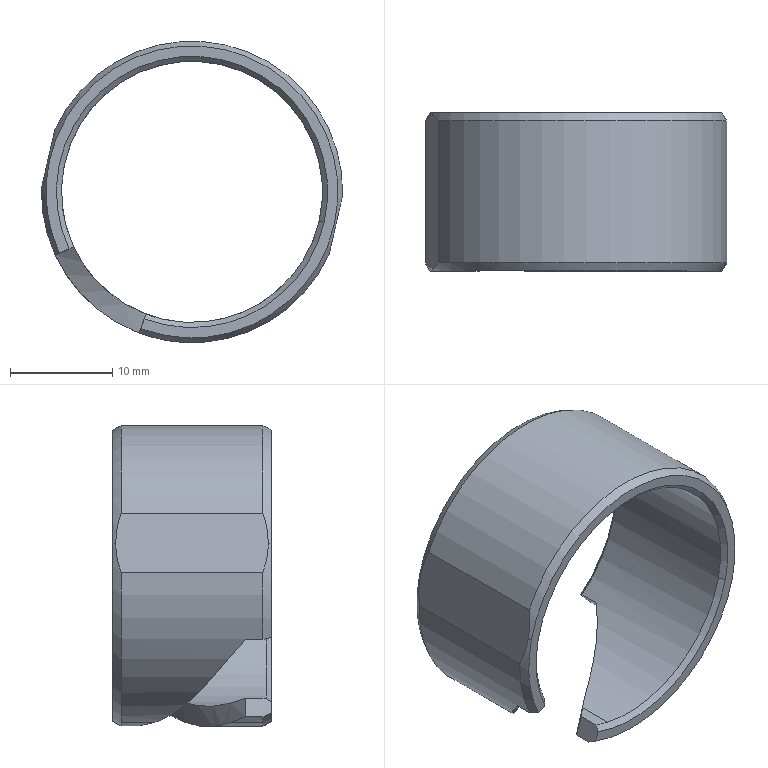Part | SolidWorks | features BaseBody 1 | 1 solid | 31 faces | box 29.5 x 15.5 x 29.5 mm | volume 2238 mm3 | cone 12 | cylinder 9 | plane 8 | spline 2 | commonest cylinder face diameters 29.5 x5 25.55 x4
STEP:
#1=CARTESIAN_POINT('',(1955.861,229.,865.451));
#2=VERTEX_POINT('',#1);
#3=CARTESIAN_POINT('',(1940.549,229.,855.861));
#4=VERTEX_POINT('',#3);
#5=CARTESIAN_POINT('',(1953.,229.,853.));
#6=DIRECTION('',(0.,-1.,0.));
#7=DIRECTION('',(0.2239,0.,0.9746));
#8=AXIS2_PLACEMENT_3D('',#5,#6,#7);
#9=CIRCLE('',#8,12.775);
#10=EDGE_CURVE('',#2,#4,#9,.T.);
#11=ORIENTED_EDGE('',*,*,#10,.T.);
#12=CARTESIAN_POINT('',(1940.062,229.5,855.973));
#13=VERTEX_POINT('',#12);
#14=CARTESIAN_POINT('',(1940.306,229.25,855.917));
#15=DIRECTION('',(-0.6891,0.7071,0.1583));
#16=VECTOR('',#15,1000.);
#17=LINE('',#14,#16);
#18=EDGE_CURVE('',#4,#13,#17,.T.);
#19=ORIENTED_EDGE('',*,*,#18,.T.);
#20=CARTESIAN_POINT('',(1955.973,229.5,865.938));
#21=VERTEX_POINT('',#20);
#22=CARTESIAN_POINT('',(1953.,229.5,853.));
#23=DIRECTION('',(0.,-1.,0.));
#24=DIRECTION('',(0.2239,0.,0.9746));
#25=AXIS2_PLACEMENT_3D('',#22,#23,#24);
#26=CIRCLE('',#25,13.275);
#27=EDGE_CURVE('',#21,#13,#26,.T.);
#28=ORIENTED_EDGE('',*,*,#27,.F.);
#29=CARTESIAN_POINT('',(1955.973,229.5,865.938));
#30=DIRECTION('',(-0.1583,-0.7071,-0.6891));
#31=VECTOR('',#30,1000.);
#32=LINE('',#29,#31);
#33=EDGE_CURVE('',#21,#2,#32,.T.);
#34=ORIENTED_EDGE('',*,*,#33,.T.);
#35=EDGE_LOOP('',(#11,#19,#28,#34));
#36=FACE_OUTER_BOUND('',#35,.T.);
#37=CARTESIAN_POINT('',(1953.,229.25,853.));
#38=DIRECTION('',(0.,1.,0.));
#39=DIRECTION('',(-0.9746,0.,0.2239));
#40=AXIS2_PLACEMENT_3D('',#37,#38,#39);
#41=CONICAL_SURFACE('',#40,13.025,0.7854);
#42=ADVANCED_FACE('',(#36),#41,.F.);
#43=CARTESIAN_POINT('',(1950.139,225.489,840.549));
#44=VERTEX_POINT('',#43);
#45=CARTESIAN_POINT('',(1941.412,216.5,847.623));
#46=VERTEX_POINT('',#45);
#47=CARTESIAN_POINT('',(1950.139,225.489,840.549));
#48=CARTESIAN_POINT('',(1949.226,224.707,840.759));
#49=CARTESIAN_POINT('',(1948.307,223.97,841.077));
#50=CARTESIAN_POINT('',(1946.969,222.878,841.727));
#51=CARTESIAN_POINT('',(1946.53,222.517,841.973));
#52=CARTESIAN_POINT('',(1945.691,221.804,842.51));
#53=CARTESIAN_POINT('',(1945.289,221.45,842.803));
#54=CARTESIAN_POINT('',(1944.523,220.739,843.43));
#55=CARTESIAN_POINT('',(1944.16,220.382,843.764));
#56=CARTESIAN_POINT('',(1943.477,219.655,844.47));
#57=CARTESIAN_POINT('',(1943.156,219.284,844.843));
#58=CARTESIAN_POINT('',(1942.27,218.141,845.999));
#59=CARTESIAN_POINT('',(1941.789,217.352,846.811));
#60=CARTESIAN_POINT('',(1941.412,216.5,847.623));
#61=B_SPLINE_CURVE_WITH_KNOTS('',3,(#47,#48,#49,#50,#51,#52,#53,#54,#55,#56,#57,#58,#59,#60),.UNSPECIFIED.,.F.,.F.,(4,2,2,2,2,2,4),(0.002262,0.005917,0.007745,0.009573,0.0114,0.01323,0.01689),.UNSPECIFIED.);
#62=EDGE_CURVE('',#44,#46,#61,.T.);
#63=ORIENTED_EDGE('',*,*,#62,.F.);
#64=CARTESIAN_POINT('',(1950.139,229.,840.549));
#65=VERTEX_POINT('',#64);
#66=CARTESIAN_POINT('',(1950.139,214.,840.549));
#67=DIRECTION('',(0.,1.,0.));
#68=VECTOR('',#67,1000.);
#69=LINE('',#66,#68);
#70=EDGE_CURVE('',#44,#65,#69,.T.);
#71=ORIENTED_EDGE('',*,*,#70,.T.);
#72=CARTESIAN_POINT('',(1953.,229.,853.));
#73=DIRECTION('',(0.,-1.,0.));
#74=DIRECTION('',(0.2239,0.,0.9746));
#75=AXIS2_PLACEMENT_3D('',#72,#73,#74);
#76=CIRCLE('',#75,12.775);
#77=EDGE_CURVE('',#4,#65,#76,.T.);
#78=ORIENTED_EDGE('',*,*,#77,.F.);
#79=ORIENTED_EDGE('',*,*,#10,.F.);
#80=CARTESIAN_POINT('',(1955.861,214.5,865.451));
#81=VERTEX_POINT('',#80);
#82=CARTESIAN_POINT('',(1955.861,214.5,865.451));
#83=DIRECTION('',(0.,1.,0.));
#84=VECTOR('',#83,1000.);
#85=LINE('',#82,#84);
#86=EDGE_CURVE('',#81,#2,#85,.T.);
#87=ORIENTED_EDGE('',*,*,#86,.F.);
#88=CARTESIAN_POINT('',(1941.412,214.5,847.623));
#89=VERTEX_POINT('',#88);
#90=CARTESIAN_POINT('',(1953.,214.5,853.));
#91=DIRECTION('',(0.,-1.,0.));
#92=DIRECTION('',(0.2239,0.,0.9746));
#93=AXIS2_PLACEMENT_3D('',#90,#91,#92);
#94=CIRCLE('',#93,12.775);
#95=EDGE_CURVE('',#81,#89,#94,.T.);
#96=ORIENTED_EDGE('',*,*,#95,.T.);
#97=CARTESIAN_POINT('',(1941.412,214.5,847.623));
#98=DIRECTION('',(0.,1.,0.));
#99=VECTOR('',#98,1000.);
#100=LINE('',#97,#99);
#101=EDGE_CURVE('',#89,#46,#100,.T.);
#102=ORIENTED_EDGE('',*,*,#101,.T.);
#103=EDGE_LOOP('',(#63,#71,#78,#79,#87,#96,#102));
#104=FACE_OUTER_BOUND('',#103,.T.);
#105=CARTESIAN_POINT('',(1953.,214.,853.));
#106=DIRECTION('',(0.,1.,0.));
#107=DIRECTION('',(-0.2239,0.,-0.9746));
#108=AXIS2_PLACEMENT_3D('',#105,#106,#107);
#109=CYLINDRICAL_SURFACE('',#108,12.775);
#110=ADVANCED_FACE('',(#104),#109,.F.);
#111=CARTESIAN_POINT('',(1939.075,229.5,856.2));
#112=VERTEX_POINT('',#111);
#113=CARTESIAN_POINT('',(1966.925,229.5,849.8));
#114=VERTEX_POINT('',#113);
#115=CARTESIAN_POINT('',(1953.,229.5,853.));
#116=DIRECTION('',(0.,1.,0.));
#117=DIRECTION('',(-0.09251,0.,-0.9957));
#118=AXIS2_PLACEMENT_3D('',#115,#116,#117);
#119=CIRCLE('',#118,14.288);
#120=EDGE_CURVE('',#112,#114,#119,.T.);
#121=ORIENTED_EDGE('',*,*,#120,.F.);
#122=CARTESIAN_POINT('',(1938.917,229.22,856.236));
#123=VERTEX_POINT('',#122);
#124=CARTESIAN_POINT('',(1938.85,229.1,856.251));
#125=DIRECTION('',(-0.4873,-0.866,0.112));
#126=VECTOR('',#125,1000.);
#127=LINE('',#124,#126);
#128=EDGE_CURVE('',#112,#123,#127,.T.);
#129=ORIENTED_EDGE('',*,*,#128,.T.);
#130=CARTESIAN_POINT('',(1939.58,228.7,859.12));
#131=VERTEX_POINT('',#130);
#132=CARTESIAN_POINT('',(1938.917,229.22,856.236));
#133=CARTESIAN_POINT('',(1939.145,229.22,857.227));
#134=CARTESIAN_POINT('',(1939.365,229.033,858.186));
#135=CARTESIAN_POINT('',(1939.58,228.7,859.12));
#136=B_SPLINE_CURVE_WITH_KNOTS('',3,(#132,#133,#134,#135),.UNSPECIFIED.,.F.,.F.,(4,4),(0.003005,0.006011),.UNSPECIFIED.);
#137=EDGE_CURVE('',#123,#131,#136,.T.);
#138=ORIENTED_EDGE('',*,*,#137,.T.);
#139=CARTESIAN_POINT('',(1967.746,228.7,852.649));
#140=VERTEX_POINT('',#139);
#141=CARTESIAN_POINT('',(1953.,228.7,853.));
#142=DIRECTION('',(0.,-1.,0.));
#143=DIRECTION('',(0.9997,0.,-0.02381));
#144=AXIS2_PLACEMENT_3D('',#141,#142,#143);
#145=CIRCLE('',#144,14.75);
#146=EDGE_CURVE('',#140,#131,#145,.T.);
#147=ORIENTED_EDGE('',*,*,#146,.F.);
#148=CARTESIAN_POINT('',(1967.083,229.22,849.764));
#149=VERTEX_POINT('',#148);
#150=CARTESIAN_POINT('',(1967.746,228.7,852.649));
#151=CARTESIAN_POINT('',(1967.531,229.033,851.715));
#152=CARTESIAN_POINT('',(1967.311,229.22,850.755));
#153=CARTESIAN_POINT('',(1967.083,229.22,849.764));
#154=B_SPLINE_CURVE_WITH_KNOTS('',3,(#150,#151,#152,#153),.UNSPECIFIED.,.F.,.F.,(4,4),(0.,0.003005),.UNSPECIFIED.);
#155=EDGE_CURVE('',#140,#149,#154,.T.);
#156=ORIENTED_EDGE('',*,*,#155,.T.);
#157=CARTESIAN_POINT('',(1967.15,229.1,849.749));
#158=DIRECTION('',(0.4873,-0.866,-0.112));
#159=VECTOR('',#158,1000.);
#160=LINE('',#157,#159);
#161=EDGE_CURVE('',#114,#149,#160,.T.);
#162=ORIENTED_EDGE('',*,*,#161,.F.);
#163=EDGE_LOOP('',(#121,#129,#138,#147,#156,#162));
#164=FACE_OUTER_BOUND('',#163,.T.);
#165=CARTESIAN_POINT('',(1953.,229.1,853.));
#166=DIRECTION('',(0.,-1.,0.));
#167=DIRECTION('',(0.9746,0.,-0.2239));
#168=AXIS2_PLACEMENT_3D('',#165,#166,#167);
#169=CONICAL_SURFACE('',#168,14.519,0.5236);
#170=ADVANCED_FACE('',(#164),#169,.T.);
#171=CARTESIAN_POINT('',(1962.036,229.5,841.932));
#172=VERTEX_POINT('',#171);
#173=CARTESIAN_POINT('',(1953.,229.5,853.));
#174=DIRECTION('',(0.,1.,0.));
#175=DIRECTION('',(-0.09251,0.,-0.9957));
#176=AXIS2_PLACEMENT_3D('',#173,#174,#175);
#177=CIRCLE('',#176,14.288);
#178=EDGE_CURVE('',#114,#172,#177,.T.);
#179=ORIENTED_EDGE('',*,*,#178,.F.);
#180=ORIENTED_EDGE('',*,*,#161,.T.);
#181=CARTESIAN_POINT('',(1966.42,228.7,846.88));
#182=VERTEX_POINT('',#181);
#183=CARTESIAN_POINT('',(1967.083,229.22,849.764));
#184=CARTESIAN_POINT('',(1966.855,229.22,848.773));
#185=CARTESIAN_POINT('',(1966.635,229.033,847.814));
#186=CARTESIAN_POINT('',(1966.42,228.7,846.88));
#187=B_SPLINE_CURVE_WITH_KNOTS('',3,(#183,#184,#185,#186),.UNSPECIFIED.,.F.,.F.,(4,4),(0.003005,0.006011),.UNSPECIFIED.);
#188=EDGE_CURVE('',#149,#182,#187,.T.);
#189=ORIENTED_EDGE('',*,*,#188,.T.);
#190=CARTESIAN_POINT('',(1962.328,228.7,841.574));
#191=VERTEX_POINT('',#190);
#192=CARTESIAN_POINT('',(1953.,228.7,853.));
#193=DIRECTION('',(0.,1.,0.));
#194=DIRECTION('',(0.9098,0.,-0.4149));
#195=AXIS2_PLACEMENT_3D('',#192,#193,#194);
#196=CIRCLE('',#195,14.75);
#197=EDGE_CURVE('',#182,#191,#196,.T.);
#198=ORIENTED_EDGE('',*,*,#197,.T.);
#199=CARTESIAN_POINT('',(1962.328,228.7,841.574));
#200=DIRECTION('',(-0.3162,0.866,0.3873));
#201=VECTOR('',#200,1000.);
#202=LINE('',#199,#201);
#203=EDGE_CURVE('',#191,#172,#202,.T.);
#204=ORIENTED_EDGE('',*,*,#203,.T.);
#205=EDGE_LOOP('',(#179,#180,#189,#198,#204));
#206=FACE_OUTER_BOUND('',#205,.T.);
#207=CARTESIAN_POINT('',(1953.,229.1,853.));
#208=DIRECTION('',(0.,-1.,0.));
#209=DIRECTION('',(0.9746,0.,-0.2239));
#210=AXIS2_PLACEMENT_3D('',#207,#208,#209);
#211=CONICAL_SURFACE('',#210,14.519,0.5236);
#212=ADVANCED_FACE('',(#206),#211,.T.);
#213=CARTESIAN_POINT('',(1949.697,225.489,838.625));
#214=VERTEX_POINT('',#213);
#215=CARTESIAN_POINT('',(1951.636,227.,838.313));
#216=VERTEX_POINT('',#215);
#217=CARTESIAN_POINT('',(1949.697,225.489,838.625));
#218=CARTESIAN_POINT('',(1950.348,225.972,838.475));
#219=CARTESIAN_POINT('',(1950.997,226.472,838.373));
#220=CARTESIAN_POINT('',(1951.636,227.,838.313));
#221=B_SPLINE_CURVE_WITH_KNOTS('',3,(#217,#218,#219,#220),.UNSPECIFIED.,.F.,.F.,(4,4),(0.01609,0.01854),.UNSPECIFIED.);
#222=EDGE_CURVE('',#214,#216,#221,.T.);
#223=ORIENTED_EDGE('',*,*,#222,.F.);
#224=CARTESIAN_POINT('',(1949.697,228.7,838.625));
#225=VERTEX_POINT('',#224);
#226=CARTESIAN_POINT('',(1949.697,214.,838.625));
#227=DIRECTION('',(0.,1.,0.));
#228=VECTOR('',#227,1000.);
#229=LINE('',#226,#228);
#230=EDGE_CURVE('',#214,#225,#229,.T.);
#231=ORIENTED_EDGE('',*,*,#230,.T.);
#232=CARTESIAN_POINT('',(1951.636,228.7,838.313));
#233=VERTEX_POINT('',#232);
#234=CARTESIAN_POINT('',(1953.,228.7,853.));
#235=DIRECTION('',(0.,-1.,0.));
#236=DIRECTION('',(-0.9997,0.,0.02381));
#237=AXIS2_PLACEMENT_3D('',#234,#235,#236);
#238=CIRCLE('',#237,14.75);
#239=EDGE_CURVE('',#225,#233,#238,.T.);
#240=ORIENTED_EDGE('',*,*,#239,.T.);
#241=CARTESIAN_POINT('',(1951.636,227.,838.313));
#242=DIRECTION('',(0.,1.,0.));
#243=VECTOR('',#242,1000.);
#244=LINE('',#241,#243);
#245=EDGE_CURVE('',#216,#233,#244,.T.);
#246=ORIENTED_EDGE('',*,*,#245,.F.);
#247=EDGE_LOOP('',(#223,#231,#240,#246));
#248=FACE_OUTER_BOUND('',#247,.T.);
#249=CARTESIAN_POINT('',(1953.,214.,853.));
#250=DIRECTION('',(0.,1.,0.));
#251=DIRECTION('',(-0.2239,0.,-0.9746));
#252=AXIS2_PLACEMENT_3D('',#249,#250,#251);
#253=CYLINDRICAL_SURFACE('',#252,14.75);
#254=ADVANCED_FACE('',(#248),#253,.T.);
#255=CARTESIAN_POINT('',(1966.42,214.8,846.88));
#256=VERTEX_POINT('',#255);
#257=CARTESIAN_POINT('',(1949.697,214.8,838.625));
#258=VERTEX_POINT('',#257);
#259=CARTESIAN_POINT('',(1953.,214.8,853.));
#260=DIRECTION('',(0.,1.,0.));
#261=DIRECTION('',(0.9098,0.,-0.4149));
#262=AXIS2_PLACEMENT_3D('',#259,#260,#261);
#263=CIRCLE('',#262,14.75);
#264=EDGE_CURVE('',#256,#258,#263,.T.);
#265=ORIENTED_EDGE('',*,*,#264,.T.);
#266=CARTESIAN_POINT('',(1949.697,218.011,838.625));
#267=VERTEX_POINT('',#266);
#268=CARTESIAN_POINT('',(1949.697,214.,838.625));
#269=DIRECTION('',(0.,1.,0.));
#270=VECTOR('',#269,1000.);
#271=LINE('',#268,#270);
#272=EDGE_CURVE('',#258,#267,#271,.T.);
#273=ORIENTED_EDGE('',*,*,#272,.T.);
#274=CARTESIAN_POINT('',(1962.328,227.,841.574));
#275=VERTEX_POINT('',#274);
#276=CARTESIAN_POINT('',(1962.328,227.,841.574));
#277=CARTESIAN_POINT('',(1961.515,226.136,840.911));
#278=CARTESIAN_POINT('',(1960.605,225.349,840.313));
#279=CARTESIAN_POINT('',(1959.117,224.219,839.567));
#280=CARTESIAN_POINT('',(1958.601,223.85,839.343));
#281=CARTESIAN_POINT('',(1957.533,223.121,838.952));
#282=CARTESIAN_POINT('',(1956.979,222.759,838.785));
#283=CARTESIAN_POINT('',(1955.309,221.691,838.387));
#284=CARTESIAN_POINT('',(1954.171,220.994,838.253));
#285=CARTESIAN_POINT('',(1952.468,219.913,838.249));
#286=CARTESIAN_POINT('',(1951.899,219.544,838.28));
#287=CARTESIAN_POINT('',(1950.778,218.79,838.407));
#288=CARTESIAN_POINT('',(1950.23,218.407,838.502));
#289=CARTESIAN_POINT('',(1949.697,218.011,838.625));
#290=B_SPLINE_CURVE_WITH_KNOTS('',3,(#276,#277,#278,#279,#280,#281,#282,#283,#284,#285,#286,#287,#288,#289),.UNSPECIFIED.,.F.,.F.,(4,2,2,2,2,2,4),(0.,0.004021,0.006032,0.008043,0.01206,0.01407,0.01609),.UNSPECIFIED.);
#291=EDGE_CURVE('',#275,#267,#290,.T.);
#292=ORIENTED_EDGE('',*,*,#291,.F.);
#293=CARTESIAN_POINT('',(1962.328,227.,841.574));
#294=DIRECTION('',(0.,1.,0.));
#295=VECTOR('',#294,1000.);
#296=LINE('',#293,#295);
#297=EDGE_CURVE('',#275,#191,#296,.T.);
#298=ORIENTED_EDGE('',*,*,#297,.T.);
#299=ORIENTED_EDGE('',*,*,#197,.F.);
#300=CARTESIAN_POINT('',(1966.42,214.8,846.88));
#301=DIRECTION('',(0.,1.,0.));
#302=VECTOR('',#301,1000.);
#303=LINE('',#300,#302);
#304=EDGE_CURVE('',#256,#182,#303,.T.);
#305=ORIENTED_EDGE('',*,*,#304,.F.);
#306=EDGE_LOOP('',(#265,#273,#292,#298,#299,#305));
#307=FACE_OUTER_BOUND('',#306,.T.);
#308=CARTESIAN_POINT('',(1953.,214.,853.));
#309=DIRECTION('',(0.,1.,0.));
#310=DIRECTION('',(-0.2239,0.,-0.9746));
#311=AXIS2_PLACEMENT_3D('',#308,#309,#310);
#312=CYLINDRICAL_SURFACE('',#311,14.75);
#313=ADVANCED_FACE('',(#307),#312,.T.);
#314=CARTESIAN_POINT('',(1950.139,214.5,840.549));
#315=VERTEX_POINT('',#314);
#316=CARTESIAN_POINT('',(1948.511,214.5,841.04));
#317=VERTEX_POINT('',#316);
#318=CARTESIAN_POINT('',(1953.,214.5,853.));
#319=DIRECTION('',(0.,1.,0.));
#320=DIRECTION('',(0.2239,0.,0.9746));
#321=AXIS2_PLACEMENT_3D('',#318,#319,#320);
#322=CIRCLE('',#321,12.775);
#323=EDGE_CURVE('',#315,#317,#322,.T.);
#324=ORIENTED_EDGE('',*,*,#323,.F.);
#325=CARTESIAN_POINT('',(1950.139,218.011,840.549));
#326=VERTEX_POINT('',#325);
#327=CARTESIAN_POINT('',(1950.139,214.,840.549));
#328=DIRECTION('',(0.,1.,0.));
#329=VECTOR('',#328,1000.);
#330=LINE('',#327,#329);
#331=EDGE_CURVE('',#315,#326,#330,.T.);
#332=ORIENTED_EDGE('',*,*,#331,.T.);
#333=CARTESIAN_POINT('',(1948.511,216.5,841.04));
#334=VERTEX_POINT('',#333);
#335=CARTESIAN_POINT('',(1948.511,216.5,841.04));
#336=CARTESIAN_POINT('',(1949.03,217.027,840.845));
#337=CARTESIAN_POINT('',(1949.574,217.528,840.679));
#338=CARTESIAN_POINT('',(1950.139,218.011,840.549));
#339=B_SPLINE_CURVE_WITH_KNOTS('',3,(#335,#336,#337,#338),.UNSPECIFIED.,.F.,.F.,(4,4),(0.,0.002262),.UNSPECIFIED.);
#340=EDGE_CURVE('',#334,#326,#339,.T.);
#341=ORIENTED_EDGE('',*,*,#340,.F.);
#342=CARTESIAN_POINT('',(1948.511,216.5,841.04));
#343=DIRECTION('',(0.,-1.,0.));
#344=VECTOR('',#343,1000.);
#345=LINE('',#342,#344);
#346=EDGE_CURVE('',#334,#317,#345,.T.);
#347=ORIENTED_EDGE('',*,*,#346,.T.);
#348=EDGE_LOOP('',(#324,#332,#341,#347));
#349=FACE_OUTER_BOUND('',#348,.T.);
#350=CARTESIAN_POINT('',(1953.,214.,853.));
#351=DIRECTION('',(0.,1.,0.));
#352=DIRECTION('',(-0.2239,0.,-0.9746));
#353=AXIS2_PLACEMENT_3D('',#350,#351,#352);
#354=CYLINDRICAL_SURFACE('',#353,12.775);
#355=ADVANCED_FACE('',(#349),#354,.F.);
#356=CARTESIAN_POINT('',(1965.451,214.5,850.139));
#357=VERTEX_POINT('',#356);
#358=CARTESIAN_POINT('',(1953.,214.5,853.));
#359=DIRECTION('',(0.,1.,0.));
#360=DIRECTION('',(0.2239,0.,0.9746));
#361=AXIS2_PLACEMENT_3D('',#358,#359,#360);
#362=CIRCLE('',#361,12.775);
#363=EDGE_CURVE('',#81,#357,#362,.T.);
#364=ORIENTED_EDGE('',*,*,#363,.T.);
#365=CARTESIAN_POINT('',(1965.938,214.,850.027));
#366=VERTEX_POINT('',#365);
#367=CARTESIAN_POINT('',(1965.694,214.25,850.083));
#368=DIRECTION('',(0.6891,-0.7071,-0.1583));
#369=VECTOR('',#368,1000.);
#370=LINE('',#367,#369);
#371=EDGE_CURVE('',#357,#366,#370,.T.);
#372=ORIENTED_EDGE('',*,*,#371,.T.);
#373=CARTESIAN_POINT('',(1955.973,214.,865.938));
#374=VERTEX_POINT('',#373);
#375=CARTESIAN_POINT('',(1953.,214.,853.));
#376=DIRECTION('',(0.,1.,0.));
#377=DIRECTION('',(0.2239,0.,0.9746));
#378=AXIS2_PLACEMENT_3D('',#375,#376,#377);
#379=CIRCLE('',#378,13.275);
#380=EDGE_CURVE('',#374,#366,#379,.T.);
#381=ORIENTED_EDGE('',*,*,#380,.F.);
#382=CARTESIAN_POINT('',(1955.861,214.5,865.451));
#383=DIRECTION('',(0.1583,-0.7071,0.6891));
#384=VECTOR('',#383,1000.);
#385=LINE('',#382,#384);
#386=EDGE_CURVE('',#81,#374,#385,.T.);
#387=ORIENTED_EDGE('',*,*,#386,.F.);
#388=EDGE_LOOP('',(#364,#372,#381,#387));
#389=FACE_OUTER_BOUND('',#388,.T.);
#390=CARTESIAN_POINT('',(1953.,214.25,853.));
#391=DIRECTION('',(0.,-1.,0.));
#392=DIRECTION('',(0.9746,0.,-0.2239));
#393=AXIS2_PLACEMENT_3D('',#390,#391,#392);
#394=CONICAL_SURFACE('',#393,13.025,0.7854);
#395=ADVANCED_FACE('',(#389),#394,.F.);
#396=CARTESIAN_POINT('',(1966.925,214.,849.8));
#397=VERTEX_POINT('',#396);
#398=CARTESIAN_POINT('',(1939.075,214.,856.2));
#399=VERTEX_POINT('',#398);
#400=CARTESIAN_POINT('',(1953.,214.,853.));
#401=DIRECTION('',(0.,-1.,0.));
#402=DIRECTION('',(-0.3514,0.,-0.9362));
#403=AXIS2_PLACEMENT_3D('',#400,#401,#402);
#404=CIRCLE('',#403,14.288);
#405=EDGE_CURVE('',#397,#399,#404,.T.);
#406=ORIENTED_EDGE('',*,*,#405,.F.);
#407=CARTESIAN_POINT('',(1967.083,214.28,849.764));
#408=VERTEX_POINT('',#407);
#409=CARTESIAN_POINT('',(1967.15,214.4,849.749));
#410=DIRECTION('',(0.4873,0.866,-0.112));
#411=VECTOR('',#410,1000.);
#412=LINE('',#409,#411);
#413=EDGE_CURVE('',#397,#408,#412,.T.);
#414=ORIENTED_EDGE('',*,*,#413,.T.);
#415=CARTESIAN_POINT('',(1967.746,214.8,852.649));
#416=VERTEX_POINT('',#415);
#417=CARTESIAN_POINT('',(1967.746,214.8,852.649));
#418=CARTESIAN_POINT('',(1967.531,214.467,851.715));
#419=CARTESIAN_POINT('',(1967.311,214.28,850.755));
#420=CARTESIAN_POINT('',(1967.083,214.28,849.764));
#421=B_SPLINE_CURVE_WITH_KNOTS('',3,(#417,#418,#419,#420),.UNSPECIFIED.,.F.,.F.,(4,4),(0.,0.003005),.UNSPECIFIED.);
#422=EDGE_CURVE('',#416,#408,#421,.T.);
#423=ORIENTED_EDGE('',*,*,#422,.F.);
#424=CARTESIAN_POINT('',(1939.58,214.8,859.12));
#425=VERTEX_POINT('',#424);
#426=CARTESIAN_POINT('',(1953.,214.8,853.));
#427=DIRECTION('',(0.,1.,0.));
#428=DIRECTION('',(-0.9098,0.,0.4149));
#429=AXIS2_PLACEMENT_3D('',#426,#427,#428);
#430=CIRCLE('',#429,14.75);
#431=EDGE_CURVE('',#425,#416,#430,.T.);
#432=ORIENTED_EDGE('',*,*,#431,.F.);
#433=CARTESIAN_POINT('',(1938.917,214.28,856.236));
#434=VERTEX_POINT('',#433);
#435=CARTESIAN_POINT('',(1938.917,214.28,856.236));
#436=CARTESIAN_POINT('',(1939.145,214.28,857.227));
#437=CARTESIAN_POINT('',(1939.365,214.467,858.186));
#438=CARTESIAN_POINT('',(1939.58,214.8,859.12));
#439=B_SPLINE_CURVE_WITH_KNOTS('',3,(#435,#436,#437,#438),.UNSPECIFIED.,.F.,.F.,(4,4),(0.003005,0.006011),.UNSPECIFIED.);
#440=EDGE_CURVE('',#434,#425,#439,.T.);
#441=ORIENTED_EDGE('',*,*,#440,.F.);
#442=CARTESIAN_POINT('',(1938.85,214.4,856.251));
#443=DIRECTION('',(-0.4873,0.866,0.112));
#444=VECTOR('',#443,1000.);
#445=LINE('',#442,#444);
#446=EDGE_CURVE('',#399,#434,#445,.T.);
#447=ORIENTED_EDGE('',*,*,#446,.F.);
#448=EDGE_LOOP('',(#406,#414,#423,#432,#441,#447));
#449=FACE_OUTER_BOUND('',#448,.T.);
#450=CARTESIAN_POINT('',(1953.,214.4,853.));
#451=DIRECTION('',(0.,1.,0.));
#452=DIRECTION('',(-0.9746,0.,0.2239));
#453=AXIS2_PLACEMENT_3D('',#450,#451,#452);
#454=CONICAL_SURFACE('',#453,14.519,0.5236);
#455=ADVANCED_FACE('',(#449),#454,.T.);
#456=CARTESIAN_POINT('',(1940.039,214.,846.986));
#457=VERTEX_POINT('',#456);
#458=CARTESIAN_POINT('',(1953.,214.,853.));
#459=DIRECTION('',(0.,-1.,0.));
#460=DIRECTION('',(-0.3514,0.,-0.9362));
#461=AXIS2_PLACEMENT_3D('',#458,#459,#460);
#462=CIRCLE('',#461,14.288);
#463=EDGE_CURVE('',#399,#457,#462,.T.);
#464=ORIENTED_EDGE('',*,*,#463,.F.);
#465=ORIENTED_EDGE('',*,*,#446,.T.);
#466=CARTESIAN_POINT('',(1938.254,214.8,853.351));
#467=VERTEX_POINT('',#466);
#468=CARTESIAN_POINT('',(1938.254,214.8,853.351));
#469=CARTESIAN_POINT('',(1938.469,214.467,854.285));
#470=CARTESIAN_POINT('',(1938.689,214.28,855.245));
#471=CARTESIAN_POINT('',(1938.917,214.28,856.236));
#472=B_SPLINE_CURVE_WITH_KNOTS('',3,(#468,#469,#470,#471),.UNSPECIFIED.,.F.,.F.,(4,4),(0.,0.003005),.UNSPECIFIED.);
#473=EDGE_CURVE('',#467,#434,#472,.T.);
#474=ORIENTED_EDGE('',*,*,#473,.F.);
#475=CARTESIAN_POINT('',(1939.62,214.8,846.792));
#476=VERTEX_POINT('',#475);
#477=CARTESIAN_POINT('',(1953.,214.8,853.));
#478=DIRECTION('',(0.,1.,0.));
#479=DIRECTION('',(-0.9071,0.,-0.4209));
#480=AXIS2_PLACEMENT_3D('',#477,#478,#479);
#481=CIRCLE('',#480,14.75);
#482=EDGE_CURVE('',#476,#467,#481,.T.);
#483=ORIENTED_EDGE('',*,*,#482,.F.);
#484=CARTESIAN_POINT('',(1940.039,214.,846.986));
#485=DIRECTION('',(-0.4536,0.866,-0.2105));
#486=VECTOR('',#485,1000.);
#487=LINE('',#484,#486);
#488=EDGE_CURVE('',#457,#476,#487,.T.);
#489=ORIENTED_EDGE('',*,*,#488,.F.);
#490=EDGE_LOOP('',(#464,#465,#474,#483,#489));
#491=FACE_OUTER_BOUND('',#490,.T.);
#492=CARTESIAN_POINT('',(1953.,214.4,853.));
#493=DIRECTION('',(0.,1.,0.));
#494=DIRECTION('',(-0.9746,0.,0.2239));
#495=AXIS2_PLACEMENT_3D('',#492,#493,#494);
#496=CONICAL_SURFACE('',#495,14.519,0.5236);
#497=ADVANCED_FACE('',(#491),#496,.T.);
#498=CARTESIAN_POINT('',(1940.958,214.,847.413));
#499=VERTEX_POINT('',#498);
#500=CARTESIAN_POINT('',(1940.958,214.,847.413));
#501=DIRECTION('',(-0.9071,0.,-0.4209));
#502=VECTOR('',#501,1000.);
#503=LINE('',#500,#502);
#504=EDGE_CURVE('',#499,#457,#503,.T.);
#505=ORIENTED_EDGE('',*,*,#504,.F.);
#506=CARTESIAN_POINT('',(1953.,214.,853.));
#507=DIRECTION('',(0.,-1.,0.));
#508=DIRECTION('',(0.2239,0.,0.9746));
#509=AXIS2_PLACEMENT_3D('',#506,#507,#508);
#510=CIRCLE('',#509,13.275);
#511=EDGE_CURVE('',#374,#499,#510,.T.);
#512=ORIENTED_EDGE('',*,*,#511,.F.);
#513=ORIENTED_EDGE('',*,*,#380,.T.);
#514=CARTESIAN_POINT('',(1948.335,214.,840.572));
#515=VERTEX_POINT('',#514);
#516=CARTESIAN_POINT('',(1953.,214.,853.));
#517=DIRECTION('',(0.,1.,0.));
#518=DIRECTION('',(0.2239,0.,0.9746));
#519=AXIS2_PLACEMENT_3D('',#516,#517,#518);
#520=CIRCLE('',#519,13.275);
#521=EDGE_CURVE('',#366,#515,#520,.T.);
#522=ORIENTED_EDGE('',*,*,#521,.T.);
#523=CARTESIAN_POINT('',(1947.979,214.,839.623));
#524=VERTEX_POINT('',#523);
#525=CARTESIAN_POINT('',(1947.979,214.,839.623));
#526=DIRECTION('',(0.3514,0.,0.9362));
#527=VECTOR('',#526,1000.);
#528=LINE('',#525,#527);
#529=EDGE_CURVE('',#524,#515,#528,.T.);
#530=ORIENTED_EDGE('',*,*,#529,.F.);
#531=CARTESIAN_POINT('',(1953.,214.,853.));
#532=DIRECTION('',(0.,-1.,0.));
#533=DIRECTION('',(-0.3514,0.,-0.9362));
#534=AXIS2_PLACEMENT_3D('',#531,#532,#533);
#535=CIRCLE('',#534,14.288);
#536=EDGE_CURVE('',#524,#397,#535,.T.);
#537=ORIENTED_EDGE('',*,*,#536,.T.);
#538=ORIENTED_EDGE('',*,*,#405,.T.);
#539=ORIENTED_EDGE('',*,*,#463,.T.);
#540=EDGE_LOOP('',(#505,#512,#513,#522,#530,#537,#538,#539));
#541=FACE_OUTER_BOUND('',#540,.T.);
#542=CARTESIAN_POINT('',(1953.,214.,853.));
#543=DIRECTION('',(0.,1.,0.));
#544=DIRECTION('',(-0.9746,0.,0.2239));
#545=AXIS2_PLACEMENT_3D('',#542,#543,#544);
#546=PLANE('',#545);
#547=ADVANCED_FACE('',(#541),#546,.F.);
#548=ORIENTED_EDGE('',*,*,#413,.F.);
#549=ORIENTED_EDGE('',*,*,#536,.F.);
#550=CARTESIAN_POINT('',(1947.817,214.8,839.191));
#551=VERTEX_POINT('',#550);
#552=CARTESIAN_POINT('',(1947.979,214.,839.623));
#553=DIRECTION('',(-0.1757,0.866,-0.4681));
#554=VECTOR('',#553,1000.);
#555=LINE('',#552,#554);
#556=EDGE_CURVE('',#524,#551,#555,.T.);
#557=ORIENTED_EDGE('',*,*,#556,.T.);
#558=CARTESIAN_POINT('',(1953.,214.8,853.));
#559=DIRECTION('',(0.,1.,0.));
#560=DIRECTION('',(0.9098,0.,-0.4149));
#561=AXIS2_PLACEMENT_3D('',#558,#559,#560);
#562=CIRCLE('',#561,14.75);
#563=EDGE_CURVE('',#258,#551,#562,.T.);
#564=ORIENTED_EDGE('',*,*,#563,.F.);
#565=ORIENTED_EDGE('',*,*,#264,.F.);
#566=CARTESIAN_POINT('',(1967.083,214.28,849.764));
#567=CARTESIAN_POINT('',(1966.855,214.28,848.773));
#568=CARTESIAN_POINT('',(1966.635,214.467,847.814));
#569=CARTESIAN_POINT('',(1966.42,214.8,846.88));
#570=B_SPLINE_CURVE_WITH_KNOTS('',3,(#566,#567,#568,#569),.UNSPECIFIED.,.F.,.F.,(4,4),(0.003005,0.006011),.UNSPECIFIED.);
#571=EDGE_CURVE('',#408,#256,#570,.T.);
#572=ORIENTED_EDGE('',*,*,#571,.F.);
#573=EDGE_LOOP('',(#548,#549,#557,#564,#565,#572));
#574=FACE_OUTER_BOUND('',#573,.T.);
#575=CARTESIAN_POINT('',(1953.,214.4,853.));
#576=DIRECTION('',(0.,1.,0.));
#577=DIRECTION('',(-0.9746,0.,0.2239));
#578=AXIS2_PLACEMENT_3D('',#575,#576,#577);
#579=CONICAL_SURFACE('',#578,14.519,0.5236);
#580=ADVANCED_FACE('',(#574),#579,.T.);
#581=CARTESIAN_POINT('',(1939.62,216.5,846.792));
#582=VERTEX_POINT('',#581);
#583=CARTESIAN_POINT('',(1939.62,216.5,846.792));
#584=DIRECTION('',(0.,-1.,0.));
#585=VECTOR('',#584,1000.);
#586=LINE('',#583,#585);
#587=EDGE_CURVE('',#582,#476,#586,.T.);
#588=ORIENTED_EDGE('',*,*,#587,.F.);
#589=CARTESIAN_POINT('',(1939.62,216.5,846.792));
#590=DIRECTION('',(0.9071,0.,0.4209));
#591=VECTOR('',#590,1000.);
#592=LINE('',#589,#591);
#593=EDGE_CURVE('',#582,#46,#592,.T.);
#594=ORIENTED_EDGE('',*,*,#593,.T.);
#595=ORIENTED_EDGE('',*,*,#101,.F.);
#596=CARTESIAN_POINT('',(1940.958,214.,847.413));
#597=DIRECTION('',(0.6414,0.7071,0.2976));
#598=VECTOR('',#597,1000.);
#599=LINE('',#596,#598);
#600=EDGE_CURVE('',#499,#89,#599,.T.);
#601=ORIENTED_EDGE('',*,*,#600,.F.);
#602=ORIENTED_EDGE('',*,*,#504,.T.);
#603=ORIENTED_EDGE('',*,*,#488,.T.);
#604=EDGE_LOOP('',(#588,#594,#595,#601,#602,#603));
#605=FACE_OUTER_BOUND('',#604,.T.);
#606=CARTESIAN_POINT('',(1941.412,214.,847.623));
#607=DIRECTION('',(-0.4209,0.,0.9071));
#608=DIRECTION('',(0.9071,0.,0.4209));
#609=AXIS2_PLACEMENT_3D('',#606,#607,#608);
#610=PLANE('',#609);
#611=ADVANCED_FACE('',(#605),#610,.F.);
#612=ORIENTED_EDGE('',*,*,#600,.T.);
#613=ORIENTED_EDGE('',*,*,#95,.F.);
#614=ORIENTED_EDGE('',*,*,#386,.T.);
#615=ORIENTED_EDGE('',*,*,#511,.T.);
#616=EDGE_LOOP('',(#612,#613,#614,#615));
#617=FACE_OUTER_BOUND('',#616,.T.);
#618=CARTESIAN_POINT('',(1953.,214.25,853.));
#619=DIRECTION('',(0.,-1.,0.));
#620=DIRECTION('',(0.9746,0.,-0.2239));
#621=AXIS2_PLACEMENT_3D('',#618,#619,#620);
#622=CONICAL_SURFACE('',#621,13.025,0.7854);
#623=ADVANCED_FACE('',(#617),#622,.F.);
#624=ORIENTED_EDGE('',*,*,#371,.F.);
#625=CARTESIAN_POINT('',(1953.,214.5,853.));
#626=DIRECTION('',(0.,1.,0.));
#627=DIRECTION('',(0.2239,0.,0.9746));
#628=AXIS2_PLACEMENT_3D('',#625,#626,#627);
#629=CIRCLE('',#628,12.775);
#630=EDGE_CURVE('',#357,#315,#629,.T.);
#631=ORIENTED_EDGE('',*,*,#630,.T.);
#632=ORIENTED_EDGE('',*,*,#323,.T.);
#633=CARTESIAN_POINT('',(1948.511,214.5,841.04));
#634=DIRECTION('',(-0.2485,-0.7071,-0.662));
#635=VECTOR('',#634,1000.);
#636=LINE('',#633,#635);
#637=EDGE_CURVE('',#317,#515,#636,.T.);
#638=ORIENTED_EDGE('',*,*,#637,.T.);
#639=ORIENTED_EDGE('',*,*,#521,.F.);
#640=EDGE_LOOP('',(#624,#631,#632,#638,#639));
#641=FACE_OUTER_BOUND('',#640,.T.);
#642=CARTESIAN_POINT('',(1953.,214.25,853.));
#643=DIRECTION('',(0.,-1.,0.));
#644=DIRECTION('',(0.9746,0.,-0.2239));
#645=AXIS2_PLACEMENT_3D('',#642,#643,#644);
#646=CONICAL_SURFACE('',#645,13.025,0.7854);
#647=ADVANCED_FACE('',(#641),#646,.F.);
#648=ORIENTED_EDGE('',*,*,#331,.F.);
#649=ORIENTED_EDGE('',*,*,#630,.F.);
#650=ORIENTED_EDGE('',*,*,#363,.F.);
#651=ORIENTED_EDGE('',*,*,#86,.T.);
#652=CARTESIAN_POINT('',(1961.079,229.,843.104));
#653=VERTEX_POINT('',#652);
#654=CARTESIAN_POINT('',(1953.,229.,853.));
#655=DIRECTION('',(0.,-1.,0.));
#656=DIRECTION('',(0.6324,0.,-0.7746));
#657=AXIS2_PLACEMENT_3D('',#654,#655,#656);
#658=CIRCLE('',#657,12.775);
#659=EDGE_CURVE('',#653,#2,#658,.T.);
#660=ORIENTED_EDGE('',*,*,#659,.F.);
#661=CARTESIAN_POINT('',(1961.079,227.,843.104));
#662=VERTEX_POINT('',#661);
#663=CARTESIAN_POINT('',(1961.079,227.,843.104));
#664=DIRECTION('',(0.,1.,0.));
#665=VECTOR('',#664,1000.);
#666=LINE('',#663,#665);
#667=EDGE_CURVE('',#662,#653,#666,.T.);
#668=ORIENTED_EDGE('',*,*,#667,.F.);
#669=CARTESIAN_POINT('',(1950.139,218.011,840.549));
#670=CARTESIAN_POINT('',(1951.052,218.793,840.34));
#671=CARTESIAN_POINT('',(1952.018,219.53,840.224));
#672=CARTESIAN_POINT('',(1953.506,220.622,840.225));
#673=CARTESIAN_POINT('',(1954.008,220.983,840.255));
#674=CARTESIAN_POINT('',(1954.997,221.696,840.372));
#675=CARTESIAN_POINT('',(1955.487,222.05,840.46));
#676=CARTESIAN_POINT('',(1956.449,222.761,840.689));
#677=CARTESIAN_POINT('',(1956.922,223.118,840.832));
#678=CARTESIAN_POINT('',(1957.845,223.845,841.169));
#679=CARTESIAN_POINT('',(1958.296,224.216,841.364));
#680=CARTESIAN_POINT('',(1959.598,225.359,842.018));
#681=CARTESIAN_POINT('',(1960.385,226.148,842.538));
#682=CARTESIAN_POINT('',(1961.079,227.,843.104));
#683=B_SPLINE_CURVE_WITH_KNOTS('',3,(#669,#670,#671,#672,#673,#674,#675,#676,#677,#678,#679,#680,#681,#682),.UNSPECIFIED.,.F.,.F.,(4,2,2,2,2,2,4),(0.002262,0.005917,0.007745,0.009573,0.0114,0.01323,0.01689),.UNSPECIFIED.);
#684=EDGE_CURVE('',#326,#662,#683,.T.);
#685=ORIENTED_EDGE('',*,*,#684,.F.);
#686=EDGE_LOOP('',(#648,#649,#650,#651,#660,#668,#685));
#687=FACE_OUTER_BOUND('',#686,.T.);
#688=CARTESIAN_POINT('',(1953.,214.,853.));
#689=DIRECTION('',(0.,1.,0.));
#690=DIRECTION('',(-0.2239,0.,-0.9746));
#691=AXIS2_PLACEMENT_3D('',#688,#689,#690);
#692=CYLINDRICAL_SURFACE('',#691,12.775);
#693=ADVANCED_FACE('',(#687),#692,.F.);
#694=ORIENTED_EDGE('',*,*,#529,.T.);
#695=ORIENTED_EDGE('',*,*,#637,.F.);
#696=ORIENTED_EDGE('',*,*,#346,.F.);
#697=CARTESIAN_POINT('',(1947.817,216.5,839.191));
#698=VERTEX_POINT('',#697);
#699=CARTESIAN_POINT('',(1948.511,216.5,841.04));
#700=DIRECTION('',(-0.3514,0.,-0.9362));
#701=VECTOR('',#700,1000.);
#702=LINE('',#699,#701);
#703=EDGE_CURVE('',#334,#698,#702,.T.);
#704=ORIENTED_EDGE('',*,*,#703,.T.);
#705=CARTESIAN_POINT('',(1947.817,214.8,839.191));
#706=DIRECTION('',(0.,1.,0.));
#707=VECTOR('',#706,1000.);
#708=LINE('',#705,#707);
#709=EDGE_CURVE('',#551,#698,#708,.T.);
#710=ORIENTED_EDGE('',*,*,#709,.F.);
#711=ORIENTED_EDGE('',*,*,#556,.F.);
#712=EDGE_LOOP('',(#694,#695,#696,#704,#710,#711));
#713=FACE_OUTER_BOUND('',#712,.T.);
#714=CARTESIAN_POINT('',(1947.817,214.,839.191));
#715=DIRECTION('',(0.9362,0.,-0.3514));
#716=DIRECTION('',(-0.3514,0.,-0.9362));
#717=AXIS2_PLACEMENT_3D('',#714,#715,#716);
#718=PLANE('',#717);
#719=ADVANCED_FACE('',(#713),#718,.F.);
#720=ORIENTED_EDGE('',*,*,#272,.F.);
#721=ORIENTED_EDGE('',*,*,#563,.T.);
#722=ORIENTED_EDGE('',*,*,#709,.T.);
#723=CARTESIAN_POINT('',(1949.697,218.011,838.625));
#724=CARTESIAN_POINT('',(1949.046,217.528,838.774));
#725=CARTESIAN_POINT('',(1948.417,217.028,838.965));
#726=CARTESIAN_POINT('',(1947.817,216.5,839.191));
#727=B_SPLINE_CURVE_WITH_KNOTS('',3,(#723,#724,#725,#726),.UNSPECIFIED.,.F.,.F.,(4,4),(0.01609,0.01854),.UNSPECIFIED.);
#728=EDGE_CURVE('',#267,#698,#727,.T.);
#729=ORIENTED_EDGE('',*,*,#728,.F.);
#730=EDGE_LOOP('',(#720,#721,#722,#729));
#731=FACE_OUTER_BOUND('',#730,.T.);
#732=CARTESIAN_POINT('',(1953.,214.,853.));
#733=DIRECTION('',(0.,1.,0.));
#734=DIRECTION('',(-0.2239,0.,-0.9746));
#735=AXIS2_PLACEMENT_3D('',#732,#733,#734);
#736=CYLINDRICAL_SURFACE('',#735,14.75);
#737=ADVANCED_FACE('',(#731),#736,.T.);
#738=ORIENTED_EDGE('',*,*,#230,.F.);
#739=CARTESIAN_POINT('',(1939.62,216.5,846.792));
#740=CARTESIAN_POINT('',(1940.062,217.364,845.84));
#741=CARTESIAN_POINT('',(1940.62,218.151,844.905));
#742=CARTESIAN_POINT('',(1941.633,219.281,843.584));
#743=CARTESIAN_POINT('',(1942.,219.65,843.157));
#744=CARTESIAN_POINT('',(1942.79,220.379,842.339));
#745=CARTESIAN_POINT('',(1943.215,220.741,841.948));
#746=CARTESIAN_POINT('',(1944.544,221.809,840.86));
#747=CARTESIAN_POINT('',(1945.509,222.506,840.243));
#748=CARTESIAN_POINT('',(1947.04,223.587,839.496));
#749=CARTESIAN_POINT('',(1947.566,223.956,839.276));
#750=CARTESIAN_POINT('',(1948.629,224.71,838.901));
#751=CARTESIAN_POINT('',(1949.164,225.093,838.747));
#752=CARTESIAN_POINT('',(1949.697,225.489,838.625));
#753=B_SPLINE_CURVE_WITH_KNOTS('',3,(#739,#740,#741,#742,#743,#744,#745,#746,#747,#748,#749,#750,#751,#752),.UNSPECIFIED.,.F.,.F.,(4,2,2,2,2,2,4),(0.,0.004021,0.006032,0.008043,0.01206,0.01407,0.01609),.UNSPECIFIED.);
#754=EDGE_CURVE('',#582,#214,#753,.T.);
#755=ORIENTED_EDGE('',*,*,#754,.F.);
#756=ORIENTED_EDGE('',*,*,#587,.T.);
#757=ORIENTED_EDGE('',*,*,#482,.T.);
#758=CARTESIAN_POINT('',(1938.254,228.7,853.351));
#759=VERTEX_POINT('',#758);
#760=CARTESIAN_POINT('',(1938.254,214.8,853.351));
#761=DIRECTION('',(0.,1.,0.));
#762=VECTOR('',#761,1000.);
#763=LINE('',#760,#762);
#764=EDGE_CURVE('',#467,#759,#763,.T.);
#765=ORIENTED_EDGE('',*,*,#764,.T.);
#766=CARTESIAN_POINT('',(1953.,228.7,853.));
#767=DIRECTION('',(0.,-1.,0.));
#768=DIRECTION('',(-0.9997,0.,0.02381));
#769=AXIS2_PLACEMENT_3D('',#766,#767,#768);
#770=CIRCLE('',#769,14.75);
#771=EDGE_CURVE('',#759,#225,#770,.T.);
#772=ORIENTED_EDGE('',*,*,#771,.T.);
#773=EDGE_LOOP('',(#738,#755,#756,#757,#765,#772));
#774=FACE_OUTER_BOUND('',#773,.T.);
#775=CARTESIAN_POINT('',(1953.,214.,853.));
#776=DIRECTION('',(0.,1.,0.));
#777=DIRECTION('',(-0.2239,0.,-0.9746));
#778=AXIS2_PLACEMENT_3D('',#775,#776,#777);
#779=CYLINDRICAL_SURFACE('',#778,14.75);
#780=ADVANCED_FACE('',(#774),#779,.T.);
#781=CARTESIAN_POINT('',(1939.58,214.8,859.12));
#782=DIRECTION('',(0.,1.,0.));
#783=VECTOR('',#782,1000.);
#784=LINE('',#781,#783);
#785=EDGE_CURVE('',#425,#131,#784,.T.);
#786=ORIENTED_EDGE('',*,*,#785,.F.);
#787=ORIENTED_EDGE('',*,*,#431,.T.);
#788=CARTESIAN_POINT('',(1967.746,214.8,852.649));
#789=DIRECTION('',(0.,1.,0.));
#790=VECTOR('',#789,1000.);
#791=LINE('',#788,#790);
#792=EDGE_CURVE('',#416,#140,#791,.T.);
#793=ORIENTED_EDGE('',*,*,#792,.T.);
#794=ORIENTED_EDGE('',*,*,#146,.T.);
#795=EDGE_LOOP('',(#786,#787,#793,#794));
#796=FACE_OUTER_BOUND('',#795,.T.);
#797=CARTESIAN_POINT('',(1953.,214.,853.));
#798=DIRECTION('',(0.,1.,0.));
#799=DIRECTION('',(-0.2239,0.,-0.9746));
#800=AXIS2_PLACEMENT_3D('',#797,#798,#799);
#801=CYLINDRICAL_SURFACE('',#800,14.75);
#802=ADVANCED_FACE('',(#796),#801,.T.);
#803=ORIENTED_EDGE('',*,*,#128,.F.);
#804=CARTESIAN_POINT('',(1951.678,229.5,838.773));
#805=VERTEX_POINT('',#804);
#806=CARTESIAN_POINT('',(1953.,229.5,853.));
#807=DIRECTION('',(0.,1.,0.));
#808=DIRECTION('',(-0.09251,0.,-0.9957));
#809=AXIS2_PLACEMENT_3D('',#806,#807,#808);
#810=CIRCLE('',#809,14.288);
#811=EDGE_CURVE('',#805,#112,#810,.T.);
#812=ORIENTED_EDGE('',*,*,#811,.F.);
#813=CARTESIAN_POINT('',(1951.636,228.7,838.313));
#814=DIRECTION('',(0.04625,0.866,0.4979));
#815=VECTOR('',#814,1000.);
#816=LINE('',#813,#815);
#817=EDGE_CURVE('',#233,#805,#816,.T.);
#818=ORIENTED_EDGE('',*,*,#817,.F.);
#819=ORIENTED_EDGE('',*,*,#239,.F.);
#820=ORIENTED_EDGE('',*,*,#771,.F.);
#821=CARTESIAN_POINT('',(1938.254,228.7,853.351));
#822=CARTESIAN_POINT('',(1938.469,229.033,854.285));
#823=CARTESIAN_POINT('',(1938.689,229.22,855.245));
#824=CARTESIAN_POINT('',(1938.917,229.22,856.236));
#825=B_SPLINE_CURVE_WITH_KNOTS('',3,(#821,#822,#823,#824),.UNSPECIFIED.,.F.,.F.,(4,4),(0.,0.003005),.UNSPECIFIED.);
#826=EDGE_CURVE('',#759,#123,#825,.T.);
#827=ORIENTED_EDGE('',*,*,#826,.T.);
#828=EDGE_LOOP('',(#803,#812,#818,#819,#820,#827));
#829=FACE_OUTER_BOUND('',#828,.T.);
#830=CARTESIAN_POINT('',(1953.,229.1,853.));
#831=DIRECTION('',(0.,-1.,0.));
#832=DIRECTION('',(0.9746,0.,-0.2239));
#833=AXIS2_PLACEMENT_3D('',#830,#831,#832);
#834=CONICAL_SURFACE('',#833,14.519,0.5236);
#835=ADVANCED_FACE('',(#829),#834,.T.);
#836=CARTESIAN_POINT('',(1951.772,229.5,839.782));
#837=VERTEX_POINT('',#836);
#838=CARTESIAN_POINT('',(1951.678,229.5,838.773));
#839=DIRECTION('',(0.09251,0.,0.9957));
#840=VECTOR('',#839,1000.);
#841=LINE('',#838,#840);
#842=EDGE_CURVE('',#805,#837,#841,.T.);
#843=ORIENTED_EDGE('',*,*,#842,.T.);
#844=CARTESIAN_POINT('',(1951.818,229.,840.28));
#845=VERTEX_POINT('',#844);
#846=CARTESIAN_POINT('',(1951.818,229.,840.28));
#847=DIRECTION('',(-0.06541,0.7071,-0.7041));
#848=VECTOR('',#847,1000.);
#849=LINE('',#846,#848);
#850=EDGE_CURVE('',#845,#837,#849,.T.);
#851=ORIENTED_EDGE('',*,*,#850,.F.);
#852=CARTESIAN_POINT('',(1951.818,227.,840.28));
#853=VERTEX_POINT('',#852);
#854=CARTESIAN_POINT('',(1951.818,227.,840.28));
#855=DIRECTION('',(0.,1.,0.));
#856=VECTOR('',#855,1000.);
#857=LINE('',#854,#856);
#858=EDGE_CURVE('',#853,#845,#857,.T.);
#859=ORIENTED_EDGE('',*,*,#858,.F.);
#860=CARTESIAN_POINT('',(1951.818,227.,840.28));
#861=DIRECTION('',(-0.09251,0.,-0.9957));
#862=VECTOR('',#861,1000.);
#863=LINE('',#860,#862);
#864=EDGE_CURVE('',#853,#216,#863,.T.);
#865=ORIENTED_EDGE('',*,*,#864,.T.);
#866=ORIENTED_EDGE('',*,*,#245,.T.);
#867=ORIENTED_EDGE('',*,*,#817,.T.);
#868=EDGE_LOOP('',(#843,#851,#859,#865,#866,#867));
#869=FACE_OUTER_BOUND('',#868,.T.);
#870=CARTESIAN_POINT('',(1951.636,229.5,838.313));
#871=DIRECTION('',(-0.9957,0.,0.09251));
#872=DIRECTION('',(0.09251,0.,0.9957));
#873=AXIS2_PLACEMENT_3D('',#870,#871,#872);
#874=PLANE('',#873);
#875=ADVANCED_FACE('',(#869),#874,.F.);
#876=ORIENTED_EDGE('',*,*,#754,.T.);
#877=ORIENTED_EDGE('',*,*,#222,.T.);
#878=ORIENTED_EDGE('',*,*,#864,.F.);
#879=CARTESIAN_POINT('',(1951.818,227.,840.28));
#880=CARTESIAN_POINT('',(1951.267,226.473,840.331));
#881=CARTESIAN_POINT('',(1950.704,225.972,840.42));
#882=CARTESIAN_POINT('',(1950.139,225.489,840.549));
#883=B_SPLINE_CURVE_WITH_KNOTS('',3,(#879,#880,#881,#882),.UNSPECIFIED.,.F.,.F.,(4,4),(0.,0.002262),.UNSPECIFIED.);
#884=EDGE_CURVE('',#853,#44,#883,.T.);
#885=ORIENTED_EDGE('',*,*,#884,.T.);
#886=ORIENTED_EDGE('',*,*,#62,.T.);
#887=ORIENTED_EDGE('',*,*,#593,.F.);
#888=EDGE_LOOP('',(#876,#877,#878,#885,#886,#887));
#889=FACE_OUTER_BOUND('',#888,.T.);
#890=CARTESIAN_POINT('',(1951.689,227.21,835.671));
#891=CARTESIAN_POINT('',(1946.83,223.57,839.099));
#892=CARTESIAN_POINT('',(1941.971,219.93,842.528));
#893=CARTESIAN_POINT('',(1937.113,216.29,845.956));
#894=CARTESIAN_POINT('',(1951.69,227.21,835.686));
#895=CARTESIAN_POINT('',(1946.835,223.57,839.111));
#896=CARTESIAN_POINT('',(1941.981,219.93,842.537));
#897=CARTESIAN_POINT('',(1937.127,216.29,845.962));
#898=CARTESIAN_POINT('',(1951.691,227.21,835.701));
#899=CARTESIAN_POINT('',(1946.841,223.57,839.123));
#900=CARTESIAN_POINT('',(1941.991,219.93,842.546));
#901=CARTESIAN_POINT('',(1937.14,216.29,845.968));
#902=CARTESIAN_POINT('',(1951.692,227.21,835.716));
#903=CARTESIAN_POINT('',(1946.846,223.57,839.136));
#904=CARTESIAN_POINT('',(1942.,219.93,842.555));
#905=CARTESIAN_POINT('',(1937.154,216.29,845.974));
#906=CARTESIAN_POINT('',(1951.753,227.21,836.525));
#907=CARTESIAN_POINT('',(1947.134,223.57,839.785));
#908=CARTESIAN_POINT('',(1942.515,219.93,843.044));
#909=CARTESIAN_POINT('',(1937.896,216.29,846.303));
#910=CARTESIAN_POINT('',(1951.82,227.21,837.408));
#911=CARTESIAN_POINT('',(1947.449,223.57,840.493));
#912=CARTESIAN_POINT('',(1943.077,219.93,843.578));
#913=CARTESIAN_POINT('',(1938.706,216.29,846.662));
#914=CARTESIAN_POINT('',(1951.898,227.21,838.438));
#915=CARTESIAN_POINT('',(1947.815,223.57,841.319));
#916=CARTESIAN_POINT('',(1943.733,219.93,844.2));
#917=CARTESIAN_POINT('',(1939.65,216.29,847.081));
#918=CARTESIAN_POINT('',(1951.932,227.21,838.88));
#919=CARTESIAN_POINT('',(1947.973,223.57,841.674));
#920=CARTESIAN_POINT('',(1944.014,219.93,844.467));
#921=CARTESIAN_POINT('',(1940.055,216.29,847.261));
#922=CARTESIAN_POINT('',(1951.971,227.21,839.396));
#923=CARTESIAN_POINT('',(1948.156,223.57,842.088));
#924=CARTESIAN_POINT('',(1944.342,219.93,844.779));
#925=CARTESIAN_POINT('',(1940.528,216.29,847.47));
#926=CARTESIAN_POINT('',(1952.004,227.21,839.838));
#927=CARTESIAN_POINT('',(1948.314,223.57,842.442));
#928=CARTESIAN_POINT('',(1944.624,219.93,845.046));
#929=CARTESIAN_POINT('',(1940.933,216.29,847.65));
#930=CARTESIAN_POINT('',(1952.024,227.21,840.1));
#931=CARTESIAN_POINT('',(1948.407,223.57,842.652));
#932=CARTESIAN_POINT('',(1944.79,219.93,845.204));
#933=CARTESIAN_POINT('',(1941.173,216.29,847.756));
#934=CARTESIAN_POINT('',(1952.032,227.21,840.213));
#935=CARTESIAN_POINT('',(1948.447,223.57,842.743));
#936=CARTESIAN_POINT('',(1944.862,219.93,845.273));
#937=CARTESIAN_POINT('',(1941.277,216.29,847.803));
#938=CARTESIAN_POINT('',(1952.036,227.21,840.254));
#939=CARTESIAN_POINT('',(1948.462,223.57,842.776));
#940=CARTESIAN_POINT('',(1944.888,219.93,845.297));
#941=CARTESIAN_POINT('',(1941.314,216.29,847.819));
#942=B_SPLINE_SURFACE_WITH_KNOTS('',3,3,((#890,#891,#892,#893),(#894,#895,#896,#897),(#898,#899,#900,#901),(#902,#903,#904,#905),(#906,#907,#908,#909),(#910,#911,#912,#913),(#914,#915,#916,#917),(#918,#919,#920,#921),(#922,#923,#924,#925),(#926,#927,#928,#929),(#930,#931,#932,#933),(#934,#935,#936,#937),(#938,#939,#940,#941)),.UNSPECIFIED.,.F.,.F.,.F.,(4,3,1,1,1,1,1,1,4),(4,4),(-0.01,0.,0.535,0.5837,0.6811,0.8272,0.9247,0.9734,1.),(0.,1.),.UNSPECIFIED.);
#943=ADVANCED_FACE('',(#889),#942,.T.);
#944=ORIENTED_EDGE('',*,*,#70,.F.);
#945=ORIENTED_EDGE('',*,*,#884,.F.);
#946=ORIENTED_EDGE('',*,*,#858,.T.);
#947=CARTESIAN_POINT('',(1953.,229.,853.));
#948=DIRECTION('',(0.,-1.,0.));
#949=DIRECTION('',(0.2239,0.,0.9746));
#950=AXIS2_PLACEMENT_3D('',#947,#948,#949);
#951=CIRCLE('',#950,12.775);
#952=EDGE_CURVE('',#65,#845,#951,.T.);
#953=ORIENTED_EDGE('',*,*,#952,.F.);
#954=EDGE_LOOP('',(#944,#945,#946,#953));
#955=FACE_OUTER_BOUND('',#954,.T.);
#956=CARTESIAN_POINT('',(1953.,214.,853.));
#957=DIRECTION('',(0.,1.,0.));
#958=DIRECTION('',(-0.2239,0.,-0.9746));
#959=AXIS2_PLACEMENT_3D('',#956,#957,#958);
#960=CYLINDRICAL_SURFACE('',#959,12.775);
#961=ADVANCED_FACE('',(#955),#960,.F.);
#962=ORIENTED_EDGE('',*,*,#18,.F.);
#963=ORIENTED_EDGE('',*,*,#77,.T.);
#964=ORIENTED_EDGE('',*,*,#952,.T.);
#965=ORIENTED_EDGE('',*,*,#850,.T.);
#966=CARTESIAN_POINT('',(1953.,229.5,853.));
#967=DIRECTION('',(0.,-1.,0.));
#968=DIRECTION('',(0.2239,0.,0.9746));
#969=AXIS2_PLACEMENT_3D('',#966,#967,#968);
#970=CIRCLE('',#969,13.275);
#971=EDGE_CURVE('',#13,#837,#970,.T.);
#972=ORIENTED_EDGE('',*,*,#971,.F.);
#973=EDGE_LOOP('',(#962,#963,#964,#965,#972));
#974=FACE_OUTER_BOUND('',#973,.T.);
#975=CARTESIAN_POINT('',(1953.,229.25,853.));
#976=DIRECTION('',(0.,1.,0.));
#977=DIRECTION('',(-0.9746,0.,0.2239));
#978=AXIS2_PLACEMENT_3D('',#975,#976,#977);
#979=CONICAL_SURFACE('',#978,13.025,0.7854);
#980=ADVANCED_FACE('',(#974),#979,.F.);
#981=CARTESIAN_POINT('',(1961.395,229.5,842.717));
#982=VERTEX_POINT('',#981);
#983=CARTESIAN_POINT('',(1961.395,229.5,842.717));
#984=DIRECTION('',(-0.4472,-0.7071,0.5477));
#985=VECTOR('',#984,1000.);
#986=LINE('',#983,#985);
#987=EDGE_CURVE('',#982,#653,#986,.T.);
#988=ORIENTED_EDGE('',*,*,#987,.T.);
#989=ORIENTED_EDGE('',*,*,#659,.T.);
#990=ORIENTED_EDGE('',*,*,#33,.F.);
#991=CARTESIAN_POINT('',(1953.,229.5,853.));
#992=DIRECTION('',(0.,-1.,0.));
#993=DIRECTION('',(0.6324,0.,-0.7746));
#994=AXIS2_PLACEMENT_3D('',#991,#992,#993);
#995=CIRCLE('',#994,13.275);
#996=EDGE_CURVE('',#982,#21,#995,.T.);
#997=ORIENTED_EDGE('',*,*,#996,.F.);
#998=EDGE_LOOP('',(#988,#989,#990,#997));
#999=FACE_OUTER_BOUND('',#998,.T.);
#1000=CARTESIAN_POINT('',(1953.,229.25,853.));
#1001=DIRECTION('',(0.,1.,0.));
#1002=DIRECTION('',(-0.9746,0.,0.2239));
#1003=AXIS2_PLACEMENT_3D('',#1000,#1001,#1002);
#1004=CONICAL_SURFACE('',#1003,13.025,0.7854);
#1005=ADVANCED_FACE('',(#999),#1004,.F.);
#1006=CARTESIAN_POINT('',(1961.395,229.5,842.717));
#1007=DIRECTION('',(0.6324,0.,-0.7746));
#1008=VECTOR('',#1007,1000.);
#1009=LINE('',#1006,#1008);
#1010=EDGE_CURVE('',#982,#172,#1009,.T.);
#1011=ORIENTED_EDGE('',*,*,#1010,.F.);
#1012=ORIENTED_EDGE('',*,*,#996,.T.);
#1013=ORIENTED_EDGE('',*,*,#27,.T.);
#1014=ORIENTED_EDGE('',*,*,#971,.T.);
#1015=ORIENTED_EDGE('',*,*,#842,.F.);
#1016=ORIENTED_EDGE('',*,*,#811,.T.);
#1017=ORIENTED_EDGE('',*,*,#120,.T.);
#1018=ORIENTED_EDGE('',*,*,#178,.T.);
#1019=EDGE_LOOP('',(#1011,#1012,#1013,#1014,#1015,#1016,#1017,#1018));
#1020=FACE_OUTER_BOUND('',#1019,.T.);
#1021=CARTESIAN_POINT('',(1953.,229.5,853.));
#1022=DIRECTION('',(0.,1.,0.));
#1023=DIRECTION('',(-0.9746,0.,0.2239));
#1024=AXIS2_PLACEMENT_3D('',#1021,#1022,#1023);
#1025=PLANE('',#1024);
#1026=ADVANCED_FACE('',(#1020),#1025,.T.);
#1027=ORIENTED_EDGE('',*,*,#297,.F.);
#1028=CARTESIAN_POINT('',(1962.328,227.,841.574));
#1029=DIRECTION('',(-0.6324,0.,0.7746));
#1030=VECTOR('',#1029,1000.);
#1031=LINE('',#1028,#1030);
#1032=EDGE_CURVE('',#275,#662,#1031,.T.);
#1033=ORIENTED_EDGE('',*,*,#1032,.T.);
#1034=ORIENTED_EDGE('',*,*,#667,.T.);
#1035=ORIENTED_EDGE('',*,*,#987,.F.);
#1036=ORIENTED_EDGE('',*,*,#1010,.T.);
#1037=ORIENTED_EDGE('',*,*,#203,.F.);
#1038=EDGE_LOOP('',(#1027,#1033,#1034,#1035,#1036,#1037));
#1039=FACE_OUTER_BOUND('',#1038,.T.);
#1040=CARTESIAN_POINT('',(1961.079,229.5,843.104));
#1041=DIRECTION('',(0.7746,0.,0.6324));
#1042=DIRECTION('',(0.6324,0.,-0.7746));
#1043=AXIS2_PLACEMENT_3D('',#1040,#1041,#1042);
#1044=PLANE('',#1043);
#1045=ADVANCED_FACE('',(#1039),#1044,.F.);
#1046=ORIENTED_EDGE('',*,*,#340,.T.);
#1047=ORIENTED_EDGE('',*,*,#684,.T.);
#1048=ORIENTED_EDGE('',*,*,#1032,.F.);
#1049=ORIENTED_EDGE('',*,*,#291,.T.);
#1050=ORIENTED_EDGE('',*,*,#728,.T.);
#1051=ORIENTED_EDGE('',*,*,#703,.F.);
#1052=EDGE_LOOP('',(#1046,#1047,#1048,#1049,#1050,#1051));
#1053=FACE_OUTER_BOUND('',#1052,.T.);
#1054=CARTESIAN_POINT('',(1961.252,227.21,843.238));
#1055=CARTESIAN_POINT('',(1956.936,223.57,842.529));
#1056=CARTESIAN_POINT('',(1952.62,219.93,841.82));
#1057=CARTESIAN_POINT('',(1948.304,216.29,841.111));
#1058=CARTESIAN_POINT('',(1961.278,227.21,843.207));
#1059=CARTESIAN_POINT('',(1956.949,223.57,842.496));
#1060=CARTESIAN_POINT('',(1952.619,219.93,841.785));
#1061=CARTESIAN_POINT('',(1948.289,216.29,841.074));
#1062=CARTESIAN_POINT('',(1961.352,227.21,843.12));
#1063=CARTESIAN_POINT('',(1956.984,223.57,842.402));
#1064=CARTESIAN_POINT('',(1952.616,219.93,841.685));
#1065=CARTESIAN_POINT('',(1948.247,216.29,840.967));
#1066=CARTESIAN_POINT('',(1961.521,227.21,842.92));
#1067=CARTESIAN_POINT('',(1957.065,223.57,842.188));
#1068=CARTESIAN_POINT('',(1952.608,219.93,841.456));
#1069=CARTESIAN_POINT('',(1948.151,216.29,840.723));
#1070=CARTESIAN_POINT('',(1961.807,227.21,842.581));
#1071=CARTESIAN_POINT('',(1957.201,223.57,841.824));
#1072=CARTESIAN_POINT('',(1952.595,219.93,841.068));
#1073=CARTESIAN_POINT('',(1947.988,216.29,840.311));
#1074=CARTESIAN_POINT('',(1962.141,227.21,842.186));
#1075=CARTESIAN_POINT('',(1957.36,223.57,841.401));
#1076=CARTESIAN_POINT('',(1952.579,219.93,840.615));
#1077=CARTESIAN_POINT('',(1947.798,216.29,839.83));
#1078=CARTESIAN_POINT('',(1962.428,227.21,841.848));
#1079=CARTESIAN_POINT('',(1957.497,223.57,841.038));
#1080=CARTESIAN_POINT('',(1952.566,219.93,840.228));
#1081=CARTESIAN_POINT('',(1947.635,216.29,839.418));
#1082=CARTESIAN_POINT('',(1963.095,227.21,841.059));
#1083=CARTESIAN_POINT('',(1957.815,223.57,840.191));
#1084=CARTESIAN_POINT('',(1952.535,219.93,839.324));
#1085=CARTESIAN_POINT('',(1947.256,216.29,838.457));
#1086=CARTESIAN_POINT('',(1963.666,227.21,840.382));
#1087=CARTESIAN_POINT('',(1958.088,223.57,839.466));
#1088=CARTESIAN_POINT('',(1952.509,219.93,838.55));
#1089=CARTESIAN_POINT('',(1946.931,216.29,837.633));
#1090=CARTESIAN_POINT('',(1964.19,227.21,839.763));
#1091=CARTESIAN_POINT('',(1958.337,223.57,838.801));
#1092=CARTESIAN_POINT('',(1952.485,219.93,837.84));
#1093=CARTESIAN_POINT('',(1946.632,216.29,836.879));
#1094=CARTESIAN_POINT('',(1964.2,227.21,839.751));
#1095=CARTESIAN_POINT('',(1958.342,223.57,838.789));
#1096=CARTESIAN_POINT('',(1952.485,219.93,837.827));
#1097=CARTESIAN_POINT('',(1946.627,216.29,836.865));
#1098=CARTESIAN_POINT('',(1964.21,227.21,839.739));
#1099=CARTESIAN_POINT('',(1958.347,223.57,838.776));
#1100=CARTESIAN_POINT('',(1952.484,219.93,837.813));
#1101=CARTESIAN_POINT('',(1946.621,216.29,836.85));
#1102=CARTESIAN_POINT('',(1964.219,227.21,839.728));
#1103=CARTESIAN_POINT('',(1958.351,223.57,838.764));
#1104=CARTESIAN_POINT('',(1952.484,219.93,837.8));
#1105=CARTESIAN_POINT('',(1946.616,216.29,836.836));
#1106=B_SPLINE_SURFACE_WITH_KNOTS('',3,3,((#1054,#1055,#1056,#1057),(#1058,#1059,#1060,#1061),(#1062,#1063,#1064,#1065),(#1066,#1067,#1068,#1069),(#1070,#1071,#1072,#1073),(#1074,#1075,#1076,#1077),(#1078,#1079,#1080,#1081),(#1082,#1083,#1084,#1085),(#1086,#1087,#1088,#1089),(#1090,#1091,#1092,#1093),(#1094,#1095,#1096,#1097),(#1098,#1099,#1100,#1101),(#1102,#1103,#1104,#1105)),.UNSPECIFIED.,.F.,.F.,.F.,(4,1,1,1,1,1,1,3,4),(4,4),(0.,0.02664,0.07535,0.1728,0.3189,0.4163,0.465,1.,1.01),(0.,1.),.UNSPECIFIED.);
#1107=ADVANCED_FACE('',(#1053),#1106,.T.);
#1108=ORIENTED_EDGE('',*,*,#792,.F.);
#1109=ORIENTED_EDGE('',*,*,#422,.T.);
#1110=ORIENTED_EDGE('',*,*,#571,.T.);
#1111=ORIENTED_EDGE('',*,*,#304,.T.);
#1112=ORIENTED_EDGE('',*,*,#188,.F.);
#1113=ORIENTED_EDGE('',*,*,#155,.F.);
#1114=EDGE_LOOP('',(#1108,#1109,#1110,#1111,#1112,#1113));
#1115=FACE_OUTER_BOUND('',#1114,.T.);
#1116=CARTESIAN_POINT('',(1966.42,231.05,846.88));
#1117=DIRECTION('',(-0.9746,0.,0.2239));
#1118=DIRECTION('',(0.,-1.,0.));
#1119=AXIS2_PLACEMENT_3D('',#1116,#1117,#1118);
#1120=PLANE('',#1119);
#1121=ADVANCED_FACE('',(#1115),#1120,.F.);
#1122=ORIENTED_EDGE('',*,*,#764,.F.);
#1123=ORIENTED_EDGE('',*,*,#473,.T.);
#1124=ORIENTED_EDGE('',*,*,#440,.T.);
#1125=ORIENTED_EDGE('',*,*,#785,.T.);
#1126=ORIENTED_EDGE('',*,*,#137,.F.);
#1127=ORIENTED_EDGE('',*,*,#826,.F.);
#1128=EDGE_LOOP('',(#1122,#1123,#1124,#1125,#1126,#1127));
#1129=FACE_OUTER_BOUND('',#1128,.T.);
#1130=CARTESIAN_POINT('',(1939.58,231.05,859.12));
#1131=DIRECTION('',(0.9746,0.,-0.2239));
#1132=DIRECTION('',(0.,1.,0.));
#1133=AXIS2_PLACEMENT_3D('',#1130,#1131,#1132);
#1134=PLANE('',#1133);
#1135=ADVANCED_FACE('',(#1129),#1134,.F.);
#1136=CLOSED_SHELL('',(#42,#110,#170,#212,#254,#313,#355,#395,#455,#497,#547,#580,#611,#623,#647,#693,#719,#737,#780,#802,#835,#875,#943,#961,#980,#1005,#1026,#1045,#1107,#1121,#1135));
#1137=MANIFOLD_SOLID_BREP('',#1136);
#1138=CARTESIAN_POINT('',(0.,0.,0.));
#1139=DIRECTION('',(0.,0.,1.));
#1140=DIRECTION('',(1.,0.,0.));
#1141=AXIS2_PLACEMENT_3D('',#1138,#1139,#1140);
#1142=(LENGTH_UNIT()NAMED_UNIT(*)SI_UNIT(.MILLI.,.METRE.));
#1143=UNCERTAINTY_MEASURE_WITH_UNIT(LENGTH_MEASURE(0.00001),#1142,'','');
#1144=(NAMED_UNIT(*)PLANE_ANGLE_UNIT()SI_UNIT($,.RADIAN.));
#1145=(NAMED_UNIT(*)SI_UNIT($,.STERADIAN.)SOLID_ANGLE_UNIT());
#1146=(GEOMETRIC_REPRESENTATION_CONTEXT(3)GLOBAL_UNCERTAINTY_ASSIGNED_CONTEXT((#1143))GLOBAL_UNIT_ASSIGNED_CONTEXT((#1142,#1144,#1145))REPRESENTATION_CONTEXT('',''));
#1147=ADVANCED_BREP_SHAPE_REPRESENTATION('',(#1137,#1141),#1146);